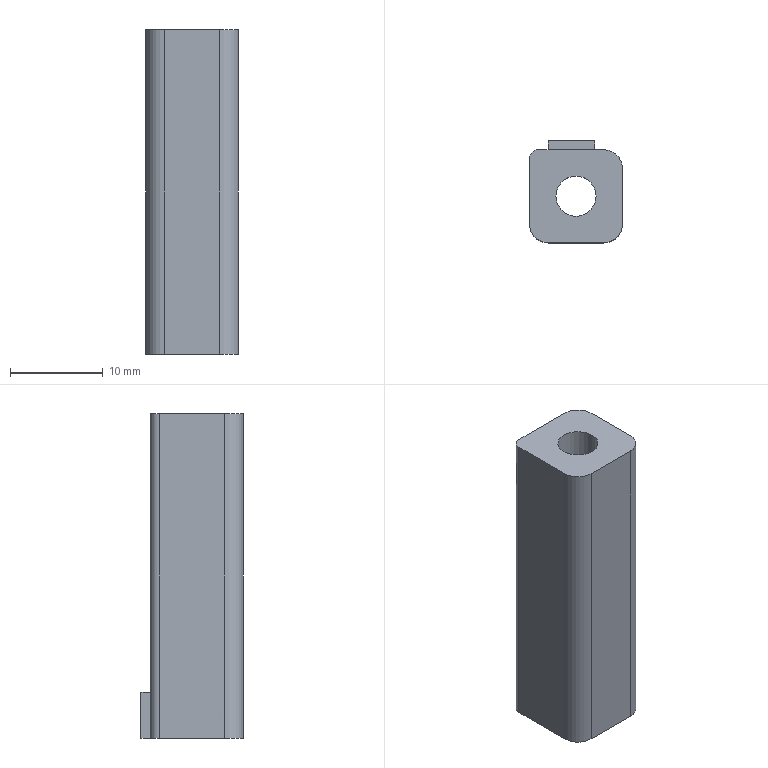Part | NX | features DIE-94 2 | 1 solid | 17 faces | box 10 x 11 x 35 mm | volume 2687 mm3 | plane 11 | cylinder 6 | commonest cylinder face diameters 4 x3 2 x1 4.32 x1 5.32 x1
STEP:
#1=CARTESIAN_POINT('',(4133.236,-872.122,828.716));
#2=VERTEX_POINT('',#1);
#3=CARTESIAN_POINT('',(4138.236,-872.122,828.716));
#4=VERTEX_POINT('',#3);
#5=CARTESIAN_POINT('',(4136.236,-872.122,828.716));
#6=DIRECTION('',(1.,0.,0.));
#7=VECTOR('',#6,1000.);
#8=LINE('',#5,#7);
#9=EDGE_CURVE('',#2,#4,#8,.T.);
#10=ORIENTED_EDGE('',*,*,#9,.F.);
#11=CARTESIAN_POINT('',(4133.236,-872.122,823.716));
#12=VERTEX_POINT('',#11);
#13=CARTESIAN_POINT('',(4133.236,-872.122,823.716));
#14=DIRECTION('',(0.,0.,-1.));
#15=VECTOR('',#14,1000.);
#16=LINE('',#13,#15);
#17=EDGE_CURVE('',#2,#12,#16,.T.);
#18=ORIENTED_EDGE('',*,*,#17,.T.);
#19=CARTESIAN_POINT('',(4132.236,-872.122,823.716));
#20=VERTEX_POINT('',#19);
#21=CARTESIAN_POINT('',(4136.236,-872.122,823.716));
#22=DIRECTION('',(-1.,0.,0.));
#23=VECTOR('',#22,1000.);
#24=LINE('',#21,#23);
#25=EDGE_CURVE('',#20,#12,#24,.F.);
#26=ORIENTED_EDGE('',*,*,#25,.F.);
#27=CARTESIAN_POINT('',(4132.236,-872.122,858.716));
#28=VERTEX_POINT('',#27);
#29=CARTESIAN_POINT('',(4132.236,-872.122,823.716));
#30=DIRECTION('',(0.,0.,1.));
#31=VECTOR('',#30,1000.);
#32=LINE('',#29,#31);
#33=EDGE_CURVE('',#20,#28,#32,.T.);
#34=ORIENTED_EDGE('',*,*,#33,.T.);
#35=CARTESIAN_POINT('',(4139.236,-872.122,858.716));
#36=VERTEX_POINT('',#35);
#37=CARTESIAN_POINT('',(4136.236,-872.122,858.716));
#38=DIRECTION('',(1.,0.,0.));
#39=VECTOR('',#38,1000.);
#40=LINE('',#37,#39);
#41=EDGE_CURVE('',#28,#36,#40,.T.);
#42=ORIENTED_EDGE('',*,*,#41,.T.);
#43=CARTESIAN_POINT('',(4139.236,-872.122,823.716));
#44=VERTEX_POINT('',#43);
#45=CARTESIAN_POINT('',(4139.236,-872.122,823.716));
#46=DIRECTION('',(0.,0.,1.));
#47=VECTOR('',#46,1000.);
#48=LINE('',#45,#47);
#49=EDGE_CURVE('',#36,#44,#48,.F.);
#50=ORIENTED_EDGE('',*,*,#49,.T.);
#51=CARTESIAN_POINT('',(4138.236,-872.122,823.716));
#52=VERTEX_POINT('',#51);
#53=CARTESIAN_POINT('',(4136.236,-872.122,823.716));
#54=DIRECTION('',(-1.,0.,0.));
#55=VECTOR('',#54,1000.);
#56=LINE('',#53,#55);
#57=EDGE_CURVE('',#52,#44,#56,.F.);
#58=ORIENTED_EDGE('',*,*,#57,.F.);
#59=CARTESIAN_POINT('',(4138.236,-872.122,823.716));
#60=DIRECTION('',(0.,0.,1.));
#61=VECTOR('',#60,1000.);
#62=LINE('',#59,#61);
#63=EDGE_CURVE('',#52,#4,#62,.T.);
#64=ORIENTED_EDGE('',*,*,#63,.T.);
#65=EDGE_LOOP('',(#10,#18,#26,#34,#42,#50,#58,#64));
#66=FACE_BOUND('',#65,.T.);
#67=CARTESIAN_POINT('',(4136.236,-872.122,823.716));
#68=DIRECTION('',(0.,1.,0.));
#69=DIRECTION('',(0.,0.,1.));
#70=AXIS2_PLACEMENT_3D('',#67,#68,#69);
#71=PLANE('',#70);
#72=ADVANCED_FACE('',(#66),#71,.T.);
#73=CARTESIAN_POINT('',(4133.576,-877.122,823.716));
#74=VERTEX_POINT('',#73);
#75=CARTESIAN_POINT('',(4136.236,-877.122,823.716));
#76=DIRECTION('',(0.,0.,-1.));
#77=DIRECTION('',(-1.,0.,0.));
#78=AXIS2_PLACEMENT_3D('',#75,#76,#77);
#79=CIRCLE('',#78,2.66);
#80=EDGE_CURVE('',#74,#74,#79,.F.);
#81=ORIENTED_EDGE('',*,*,#80,.F.);
#82=CARTESIAN_POINT('',(4133.576,-877.122,853.716));
#83=VERTEX_POINT('',#82);
#84=CARTESIAN_POINT('',(4133.576,-877.122,862.216));
#85=DIRECTION('',(0.,0.,-1.));
#86=VECTOR('',#85,1000.);
#87=LINE('',#84,#86);
#88=EDGE_CURVE('',#83,#74,#87,.T.);
#89=ORIENTED_EDGE('',*,*,#88,.F.);
#90=CARTESIAN_POINT('',(4136.236,-877.122,853.716));
#91=DIRECTION('',(0.,0.,1.));
#92=DIRECTION('',(1.,0.,0.));
#93=AXIS2_PLACEMENT_3D('',#90,#91,#92);
#94=CIRCLE('',#93,2.66);
#95=EDGE_CURVE('',#83,#83,#94,.T.);
#96=ORIENTED_EDGE('',*,*,#95,.T.);
#97=ORIENTED_EDGE('',*,*,#88,.T.);
#98=EDGE_LOOP('',(#81,#89,#96,#97));
#99=FACE_BOUND('',#98,.T.);
#100=CARTESIAN_POINT('',(4136.236,-877.122,862.216));
#101=DIRECTION('',(0.,0.,-1.));
#102=DIRECTION('',(-1.,0.,0.));
#103=AXIS2_PLACEMENT_3D('',#100,#101,#102);
#104=CYLINDRICAL_SURFACE('',#103,2.66);
#105=ADVANCED_FACE('',(#99),#104,.F.);
#106=ORIENTED_EDGE('',*,*,#25,.T.);
#107=CARTESIAN_POINT('',(4133.236,-871.122,823.716));
#108=VERTEX_POINT('',#107);
#109=CARTESIAN_POINT('',(4133.236,-871.122,823.716));
#110=DIRECTION('',(0.,-1.,0.));
#111=VECTOR('',#110,1000.);
#112=LINE('',#109,#111);
#113=EDGE_CURVE('',#108,#12,#112,.T.);
#114=ORIENTED_EDGE('',*,*,#113,.F.);
#115=CARTESIAN_POINT('',(4138.236,-871.122,823.716));
#116=VERTEX_POINT('',#115);
#117=CARTESIAN_POINT('',(4139.236,-871.122,823.716));
#118=DIRECTION('',(-1.,0.,0.));
#119=VECTOR('',#118,1000.);
#120=LINE('',#117,#119);
#121=EDGE_CURVE('',#116,#108,#120,.T.);
#122=ORIENTED_EDGE('',*,*,#121,.F.);
#123=CARTESIAN_POINT('',(4138.236,-872.172,823.716));
#124=DIRECTION('',(0.,1.,0.));
#125=VECTOR('',#124,1000.);
#126=LINE('',#123,#125);
#127=EDGE_CURVE('',#52,#116,#126,.T.);
#128=ORIENTED_EDGE('',*,*,#127,.F.);
#129=ORIENTED_EDGE('',*,*,#57,.T.);
#130=CARTESIAN_POINT('',(4141.236,-874.122,823.716));
#131=VERTEX_POINT('',#130);
#132=CARTESIAN_POINT('',(4139.236,-874.122,823.716));
#133=DIRECTION('',(0.,0.,-1.));
#134=DIRECTION('',(-1.,0.,0.));
#135=AXIS2_PLACEMENT_3D('',#132,#133,#134);
#136=CIRCLE('',#135,2.);
#137=EDGE_CURVE('',#131,#44,#136,.F.);
#138=ORIENTED_EDGE('',*,*,#137,.F.);
#139=CARTESIAN_POINT('',(4141.236,-880.122,823.716));
#140=VERTEX_POINT('',#139);
#141=CARTESIAN_POINT('',(4141.236,-877.122,823.716));
#142=DIRECTION('',(0.,1.,0.));
#143=VECTOR('',#142,1000.);
#144=LINE('',#141,#143);
#145=EDGE_CURVE('',#140,#131,#144,.T.);
#146=ORIENTED_EDGE('',*,*,#145,.F.);
#147=CARTESIAN_POINT('',(4139.236,-882.122,823.716));
#148=VERTEX_POINT('',#147);
#149=CARTESIAN_POINT('',(4139.236,-880.122,823.716));
#150=DIRECTION('',(0.,0.,-1.));
#151=DIRECTION('',(-1.,0.,0.));
#152=AXIS2_PLACEMENT_3D('',#149,#150,#151);
#153=CIRCLE('',#152,2.);
#154=EDGE_CURVE('',#148,#140,#153,.F.);
#155=ORIENTED_EDGE('',*,*,#154,.F.);
#156=CARTESIAN_POINT('',(4133.236,-882.122,823.716));
#157=VERTEX_POINT('',#156);
#158=CARTESIAN_POINT('',(4136.236,-882.122,823.716));
#159=DIRECTION('',(1.,0.,0.));
#160=VECTOR('',#159,1000.);
#161=LINE('',#158,#160);
#162=EDGE_CURVE('',#157,#148,#161,.T.);
#163=ORIENTED_EDGE('',*,*,#162,.F.);
#164=CARTESIAN_POINT('',(4131.236,-880.122,823.716));
#165=VERTEX_POINT('',#164);
#166=CARTESIAN_POINT('',(4133.236,-880.122,823.716));
#167=DIRECTION('',(0.,0.,-1.));
#168=DIRECTION('',(-1.,0.,0.));
#169=AXIS2_PLACEMENT_3D('',#166,#167,#168);
#170=CIRCLE('',#169,2.);
#171=EDGE_CURVE('',#165,#157,#170,.F.);
#172=ORIENTED_EDGE('',*,*,#171,.F.);
#173=CARTESIAN_POINT('',(4131.236,-873.122,823.716));
#174=VERTEX_POINT('',#173);
#175=CARTESIAN_POINT('',(4131.236,-877.122,823.716));
#176=DIRECTION('',(0.,-1.,0.));
#177=VECTOR('',#176,1000.);
#178=LINE('',#175,#177);
#179=EDGE_CURVE('',#174,#165,#178,.T.);
#180=ORIENTED_EDGE('',*,*,#179,.F.);
#181=CARTESIAN_POINT('',(4132.236,-873.122,823.716));
#182=DIRECTION('',(0.,0.,-1.));
#183=DIRECTION('',(-1.,0.,0.));
#184=AXIS2_PLACEMENT_3D('',#181,#182,#183);
#185=CIRCLE('',#184,1.);
#186=EDGE_CURVE('',#174,#20,#185,.T.);
#187=ORIENTED_EDGE('',*,*,#186,.T.);
#188=EDGE_LOOP('',(#106,#114,#122,#128,#129,#138,#146,#155,#163,#172,#180,#187));
#189=FACE_BOUND('',#188,.T.);
#190=ORIENTED_EDGE('',*,*,#80,.T.);
#191=EDGE_LOOP('',(#190));
#192=FACE_BOUND('',#191,.T.);
#193=CARTESIAN_POINT('',(4123.586,-858.122,823.716));
#194=DIRECTION('',(0.,0.,-1.));
#195=DIRECTION('',(-1.,0.,0.));
#196=AXIS2_PLACEMENT_3D('',#193,#194,#195);
#197=PLANE('',#196);
#198=ADVANCED_FACE('',(#189,#192),#197,.T.);
#199=ORIENTED_EDGE('',*,*,#95,.F.);
#200=EDGE_LOOP('',(#199));
#201=FACE_BOUND('',#200,.T.);
#202=CARTESIAN_POINT('',(4134.076,-877.122,853.716));
#203=VERTEX_POINT('',#202);
#204=CARTESIAN_POINT('',(4136.236,-877.122,853.716));
#205=DIRECTION('',(0.,0.,1.));
#206=DIRECTION('',(1.,0.,0.));
#207=AXIS2_PLACEMENT_3D('',#204,#205,#206);
#208=CIRCLE('',#207,2.16);
#209=EDGE_CURVE('',#203,#203,#208,.F.);
#210=ORIENTED_EDGE('',*,*,#209,.F.);
#211=EDGE_LOOP('',(#210));
#212=FACE_BOUND('',#211,.T.);
#213=CARTESIAN_POINT('',(4079.736,-858.122,853.716));
#214=DIRECTION('',(0.,0.,1.));
#215=DIRECTION('',(1.,0.,0.));
#216=AXIS2_PLACEMENT_3D('',#213,#214,#215);
#217=PLANE('',#216);
#218=ADVANCED_FACE('',(#201,#212),#217,.F.);
#219=CARTESIAN_POINT('',(4134.076,-877.122,858.716));
#220=VERTEX_POINT('',#219);
#221=CARTESIAN_POINT('',(4134.076,-877.122,862.216));
#222=DIRECTION('',(0.,0.,-1.));
#223=VECTOR('',#222,1000.);
#224=LINE('',#221,#223);
#225=EDGE_CURVE('',#220,#203,#224,.T.);
#226=ORIENTED_EDGE('',*,*,#225,.T.);
#227=ORIENTED_EDGE('',*,*,#209,.T.);
#228=ORIENTED_EDGE('',*,*,#225,.F.);
#229=CARTESIAN_POINT('',(4136.236,-877.122,858.716));
#230=DIRECTION('',(0.,0.,1.));
#231=DIRECTION('',(1.,0.,0.));
#232=AXIS2_PLACEMENT_3D('',#229,#230,#231);
#233=CIRCLE('',#232,2.16);
#234=EDGE_CURVE('',#220,#220,#233,.T.);
#235=ORIENTED_EDGE('',*,*,#234,.T.);
#236=EDGE_LOOP('',(#226,#227,#228,#235));
#237=FACE_BOUND('',#236,.T.);
#238=CARTESIAN_POINT('',(4136.236,-877.122,862.216));
#239=DIRECTION('',(0.,0.,-1.));
#240=DIRECTION('',(-1.,0.,0.));
#241=AXIS2_PLACEMENT_3D('',#238,#239,#240);
#242=CYLINDRICAL_SURFACE('',#241,2.16);
#243=ADVANCED_FACE('',(#237),#242,.F.);
#244=ORIENTED_EDGE('',*,*,#234,.F.);
#245=EDGE_LOOP('',(#244));
#246=FACE_BOUND('',#245,.T.);
#247=CARTESIAN_POINT('',(4131.236,-880.122,858.716));
#248=VERTEX_POINT('',#247);
#249=CARTESIAN_POINT('',(4131.236,-873.122,858.716));
#250=VERTEX_POINT('',#249);
#251=CARTESIAN_POINT('',(4131.236,-877.122,858.716));
#252=DIRECTION('',(0.,1.,0.));
#253=VECTOR('',#252,1000.);
#254=LINE('',#251,#253);
#255=EDGE_CURVE('',#248,#250,#254,.T.);
#256=ORIENTED_EDGE('',*,*,#255,.F.);
#257=CARTESIAN_POINT('',(4133.236,-882.122,858.716));
#258=VERTEX_POINT('',#257);
#259=CARTESIAN_POINT('',(4133.236,-880.122,858.716));
#260=DIRECTION('',(0.,0.,1.));
#261=DIRECTION('',(1.,0.,0.));
#262=AXIS2_PLACEMENT_3D('',#259,#260,#261);
#263=CIRCLE('',#262,2.);
#264=EDGE_CURVE('',#258,#248,#263,.F.);
#265=ORIENTED_EDGE('',*,*,#264,.F.);
#266=CARTESIAN_POINT('',(4139.236,-882.122,858.716));
#267=VERTEX_POINT('',#266);
#268=CARTESIAN_POINT('',(4136.236,-882.122,858.716));
#269=DIRECTION('',(-1.,0.,0.));
#270=VECTOR('',#269,1000.);
#271=LINE('',#268,#270);
#272=EDGE_CURVE('',#267,#258,#271,.T.);
#273=ORIENTED_EDGE('',*,*,#272,.F.);
#274=CARTESIAN_POINT('',(4141.236,-880.122,858.716));
#275=VERTEX_POINT('',#274);
#276=CARTESIAN_POINT('',(4139.236,-880.122,858.716));
#277=DIRECTION('',(0.,0.,1.));
#278=DIRECTION('',(1.,0.,0.));
#279=AXIS2_PLACEMENT_3D('',#276,#277,#278);
#280=CIRCLE('',#279,2.);
#281=EDGE_CURVE('',#267,#275,#280,.T.);
#282=ORIENTED_EDGE('',*,*,#281,.T.);
#283=CARTESIAN_POINT('',(4141.236,-874.122,858.716));
#284=VERTEX_POINT('',#283);
#285=CARTESIAN_POINT('',(4141.236,-877.122,858.716));
#286=DIRECTION('',(0.,-1.,0.));
#287=VECTOR('',#286,1000.);
#288=LINE('',#285,#287);
#289=EDGE_CURVE('',#284,#275,#288,.T.);
#290=ORIENTED_EDGE('',*,*,#289,.F.);
#291=CARTESIAN_POINT('',(4139.236,-874.122,858.716));
#292=DIRECTION('',(0.,0.,1.));
#293=DIRECTION('',(1.,0.,0.));
#294=AXIS2_PLACEMENT_3D('',#291,#292,#293);
#295=CIRCLE('',#294,2.);
#296=EDGE_CURVE('',#284,#36,#295,.T.);
#297=ORIENTED_EDGE('',*,*,#296,.T.);
#298=ORIENTED_EDGE('',*,*,#41,.F.);
#299=CARTESIAN_POINT('',(4132.236,-873.122,858.716));
#300=DIRECTION('',(0.,0.,1.));
#301=DIRECTION('',(1.,0.,0.));
#302=AXIS2_PLACEMENT_3D('',#299,#300,#301);
#303=CIRCLE('',#302,1.);
#304=EDGE_CURVE('',#250,#28,#303,.F.);
#305=ORIENTED_EDGE('',*,*,#304,.F.);
#306=EDGE_LOOP('',(#256,#265,#273,#282,#290,#297,#298,#305));
#307=FACE_BOUND('',#306,.T.);
#308=CARTESIAN_POINT('',(4123.586,-858.122,858.716));
#309=DIRECTION('',(0.,0.,1.));
#310=DIRECTION('',(-1.,0.,0.));
#311=AXIS2_PLACEMENT_3D('',#308,#309,#310);
#312=PLANE('',#311);
#313=ADVANCED_FACE('',(#246,#307),#312,.T.);
#314=ORIENTED_EDGE('',*,*,#186,.F.);
#315=CARTESIAN_POINT('',(4131.236,-873.122,823.716));
#316=DIRECTION('',(0.,0.,1.));
#317=VECTOR('',#316,1000.);
#318=LINE('',#315,#317);
#319=EDGE_CURVE('',#250,#174,#318,.F.);
#320=ORIENTED_EDGE('',*,*,#319,.F.);
#321=ORIENTED_EDGE('',*,*,#304,.T.);
#322=ORIENTED_EDGE('',*,*,#33,.F.);
#323=EDGE_LOOP('',(#314,#320,#321,#322));
#324=FACE_BOUND('',#323,.T.);
#325=CARTESIAN_POINT('',(4132.236,-873.122,823.716));
#326=DIRECTION('',(0.,0.,1.));
#327=DIRECTION('',(1.,0.,0.));
#328=AXIS2_PLACEMENT_3D('',#325,#326,#327);
#329=CYLINDRICAL_SURFACE('',#328,1.);
#330=ADVANCED_FACE('',(#324),#329,.T.);
#331=ORIENTED_EDGE('',*,*,#171,.T.);
#332=CARTESIAN_POINT('',(4133.236,-882.122,823.716));
#333=DIRECTION('',(0.,0.,1.));
#334=VECTOR('',#333,1000.);
#335=LINE('',#332,#334);
#336=EDGE_CURVE('',#258,#157,#335,.F.);
#337=ORIENTED_EDGE('',*,*,#336,.F.);
#338=ORIENTED_EDGE('',*,*,#264,.T.);
#339=CARTESIAN_POINT('',(4131.236,-880.122,823.716));
#340=DIRECTION('',(0.,0.,1.));
#341=VECTOR('',#340,1000.);
#342=LINE('',#339,#341);
#343=EDGE_CURVE('',#165,#248,#342,.T.);
#344=ORIENTED_EDGE('',*,*,#343,.F.);
#345=EDGE_LOOP('',(#331,#337,#338,#344));
#346=FACE_BOUND('',#345,.T.);
#347=CARTESIAN_POINT('',(4133.236,-880.122,823.716));
#348=DIRECTION('',(0.,0.,1.));
#349=DIRECTION('',(1.,0.,0.));
#350=AXIS2_PLACEMENT_3D('',#347,#348,#349);
#351=CYLINDRICAL_SURFACE('',#350,2.);
#352=ADVANCED_FACE('',(#346),#351,.T.);
#353=ORIENTED_EDGE('',*,*,#154,.T.);
#354=CARTESIAN_POINT('',(4141.236,-880.122,823.716));
#355=DIRECTION('',(0.,0.,1.));
#356=VECTOR('',#355,1000.);
#357=LINE('',#354,#356);
#358=EDGE_CURVE('',#275,#140,#357,.F.);
#359=ORIENTED_EDGE('',*,*,#358,.F.);
#360=ORIENTED_EDGE('',*,*,#281,.F.);
#361=CARTESIAN_POINT('',(4139.236,-882.122,823.716));
#362=DIRECTION('',(0.,0.,1.));
#363=VECTOR('',#362,1000.);
#364=LINE('',#361,#363);
#365=EDGE_CURVE('',#148,#267,#364,.T.);
#366=ORIENTED_EDGE('',*,*,#365,.F.);
#367=EDGE_LOOP('',(#353,#359,#360,#366));
#368=FACE_BOUND('',#367,.T.);
#369=CARTESIAN_POINT('',(4139.236,-880.122,823.716));
#370=DIRECTION('',(0.,0.,1.));
#371=DIRECTION('',(1.,0.,0.));
#372=AXIS2_PLACEMENT_3D('',#369,#370,#371);
#373=CYLINDRICAL_SURFACE('',#372,2.);
#374=ADVANCED_FACE('',(#368),#373,.T.);
#375=ORIENTED_EDGE('',*,*,#137,.T.);
#376=ORIENTED_EDGE('',*,*,#49,.F.);
#377=ORIENTED_EDGE('',*,*,#296,.F.);
#378=CARTESIAN_POINT('',(4141.236,-874.122,823.716));
#379=DIRECTION('',(0.,0.,1.));
#380=VECTOR('',#379,1000.);
#381=LINE('',#378,#380);
#382=EDGE_CURVE('',#131,#284,#381,.T.);
#383=ORIENTED_EDGE('',*,*,#382,.F.);
#384=EDGE_LOOP('',(#375,#376,#377,#383));
#385=FACE_BOUND('',#384,.T.);
#386=CARTESIAN_POINT('',(4139.236,-874.122,823.716));
#387=DIRECTION('',(0.,0.,1.));
#388=DIRECTION('',(1.,0.,0.));
#389=AXIS2_PLACEMENT_3D('',#386,#387,#388);
#390=CYLINDRICAL_SURFACE('',#389,2.);
#391=ADVANCED_FACE('',(#385),#390,.T.);
#392=ORIENTED_EDGE('',*,*,#145,.T.);
#393=ORIENTED_EDGE('',*,*,#382,.T.);
#394=ORIENTED_EDGE('',*,*,#289,.T.);
#395=ORIENTED_EDGE('',*,*,#358,.T.);
#396=EDGE_LOOP('',(#392,#393,#394,#395));
#397=FACE_BOUND('',#396,.T.);
#398=CARTESIAN_POINT('',(4141.236,-877.122,823.716));
#399=DIRECTION('',(1.,0.,0.));
#400=DIRECTION('',(0.,0.,-1.));
#401=AXIS2_PLACEMENT_3D('',#398,#399,#400);
#402=PLANE('',#401);
#403=ADVANCED_FACE('',(#397),#402,.T.);
#404=ORIENTED_EDGE('',*,*,#255,.T.);
#405=ORIENTED_EDGE('',*,*,#319,.T.);
#406=ORIENTED_EDGE('',*,*,#179,.T.);
#407=ORIENTED_EDGE('',*,*,#343,.T.);
#408=EDGE_LOOP('',(#404,#405,#406,#407));
#409=FACE_BOUND('',#408,.T.);
#410=CARTESIAN_POINT('',(4131.236,-877.122,823.716));
#411=DIRECTION('',(-1.,0.,0.));
#412=DIRECTION('',(0.,0.,1.));
#413=AXIS2_PLACEMENT_3D('',#410,#411,#412);
#414=PLANE('',#413);
#415=ADVANCED_FACE('',(#409),#414,.T.);
#416=ORIENTED_EDGE('',*,*,#162,.T.);
#417=ORIENTED_EDGE('',*,*,#365,.T.);
#418=ORIENTED_EDGE('',*,*,#272,.T.);
#419=ORIENTED_EDGE('',*,*,#336,.T.);
#420=EDGE_LOOP('',(#416,#417,#418,#419));
#421=FACE_BOUND('',#420,.T.);
#422=CARTESIAN_POINT('',(4136.236,-882.122,823.716));
#423=DIRECTION('',(0.,-1.,0.));
#424=DIRECTION('',(0.,0.,-1.));
#425=AXIS2_PLACEMENT_3D('',#422,#423,#424);
#426=PLANE('',#425);
#427=ADVANCED_FACE('',(#421),#426,.T.);
#428=ORIENTED_EDGE('',*,*,#17,.F.);
#429=CARTESIAN_POINT('',(4133.236,-871.122,828.716));
#430=VERTEX_POINT('',#429);
#431=CARTESIAN_POINT('',(4133.236,-871.122,828.716));
#432=DIRECTION('',(0.,-1.,0.));
#433=VECTOR('',#432,1000.);
#434=LINE('',#431,#433);
#435=EDGE_CURVE('',#430,#2,#434,.T.);
#436=ORIENTED_EDGE('',*,*,#435,.F.);
#437=CARTESIAN_POINT('',(4133.236,-871.122,828.716));
#438=DIRECTION('',(0.,0.,-1.));
#439=VECTOR('',#438,1000.);
#440=LINE('',#437,#439);
#441=EDGE_CURVE('',#430,#108,#440,.T.);
#442=ORIENTED_EDGE('',*,*,#441,.T.);
#443=ORIENTED_EDGE('',*,*,#113,.T.);
#444=EDGE_LOOP('',(#428,#436,#442,#443));
#445=FACE_BOUND('',#444,.T.);
#446=CARTESIAN_POINT('',(4133.236,-871.122,828.716));
#447=DIRECTION('',(1.,0.,0.));
#448=DIRECTION('',(0.,0.,-1.));
#449=AXIS2_PLACEMENT_3D('',#446,#447,#448);
#450=PLANE('',#449);
#451=ADVANCED_FACE('',(#445),#450,.F.);
#452=ORIENTED_EDGE('',*,*,#63,.F.);
#453=ORIENTED_EDGE('',*,*,#127,.T.);
#454=CARTESIAN_POINT('',(4138.236,-871.122,828.716));
#455=VERTEX_POINT('',#454);
#456=CARTESIAN_POINT('',(4138.236,-871.122,828.716));
#457=DIRECTION('',(0.,0.,-1.));
#458=VECTOR('',#457,1000.);
#459=LINE('',#456,#458);
#460=EDGE_CURVE('',#455,#116,#459,.T.);
#461=ORIENTED_EDGE('',*,*,#460,.F.);
#462=CARTESIAN_POINT('',(4138.236,-872.172,828.716));
#463=DIRECTION('',(0.,1.,0.));
#464=VECTOR('',#463,1000.);
#465=LINE('',#462,#464);
#466=EDGE_CURVE('',#4,#455,#465,.T.);
#467=ORIENTED_EDGE('',*,*,#466,.F.);
#468=EDGE_LOOP('',(#452,#453,#461,#467));
#469=FACE_BOUND('',#468,.T.);
#470=CARTESIAN_POINT('',(4138.236,-872.172,828.716));
#471=DIRECTION('',(-1.,0.,0.));
#472=DIRECTION('',(0.,0.,1.));
#473=AXIS2_PLACEMENT_3D('',#470,#471,#472);
#474=PLANE('',#473);
#475=ADVANCED_FACE('',(#469),#474,.F.);
#476=ORIENTED_EDGE('',*,*,#121,.T.);
#477=ORIENTED_EDGE('',*,*,#441,.F.);
#478=CARTESIAN_POINT('',(4139.236,-871.122,828.716));
#479=DIRECTION('',(-1.,0.,0.));
#480=VECTOR('',#479,1000.);
#481=LINE('',#478,#480);
#482=EDGE_CURVE('',#455,#430,#481,.T.);
#483=ORIENTED_EDGE('',*,*,#482,.F.);
#484=ORIENTED_EDGE('',*,*,#460,.T.);
#485=EDGE_LOOP('',(#476,#477,#483,#484));
#486=FACE_BOUND('',#485,.T.);
#487=CARTESIAN_POINT('',(4139.236,-871.122,828.716));
#488=DIRECTION('',(0.,-1.,0.));
#489=DIRECTION('',(0.,0.,-1.));
#490=AXIS2_PLACEMENT_3D('',#487,#488,#489);
#491=PLANE('',#490);
#492=ADVANCED_FACE('',(#486),#491,.F.);
#493=ORIENTED_EDGE('',*,*,#435,.T.);
#494=ORIENTED_EDGE('',*,*,#9,.T.);
#495=ORIENTED_EDGE('',*,*,#466,.T.);
#496=ORIENTED_EDGE('',*,*,#482,.T.);
#497=EDGE_LOOP('',(#493,#494,#495,#496));
#498=FACE_BOUND('',#497,.T.);
#499=CARTESIAN_POINT('',(0.,0.,828.716));
#500=DIRECTION('',(0.,0.,1.));
#501=DIRECTION('',(1.,0.,0.));
#502=AXIS2_PLACEMENT_3D('',#499,#500,#501);
#503=PLANE('',#502);
#504=ADVANCED_FACE('',(#498),#503,.T.);
#505=CLOSED_SHELL('',(#72,#105,#198,#218,#243,#313,#330,#352,#374,#391,#403,#415,#427,#451,#475,#492,#504));
#506=MANIFOLD_SOLID_BREP('',#505);
#507=(LENGTH_UNIT()NAMED_UNIT(*)SI_UNIT(.MILLI.,.METRE.));
#508=UNCERTAINTY_MEASURE_WITH_UNIT(LENGTH_MEASURE(0.00001),#507,'','');
#509=(NAMED_UNIT(*)PLANE_ANGLE_UNIT()SI_UNIT($,.RADIAN.));
#510=(NAMED_UNIT(*)SI_UNIT($,.STERADIAN.)SOLID_ANGLE_UNIT());
#511=(GEOMETRIC_REPRESENTATION_CONTEXT(3)GLOBAL_UNCERTAINTY_ASSIGNED_CONTEXT((#508))GLOBAL_UNIT_ASSIGNED_CONTEXT((#507,#509,#510))REPRESENTATION_CONTEXT('',''));
#512=ADVANCED_BREP_SHAPE_REPRESENTATION('',(#506),#511);